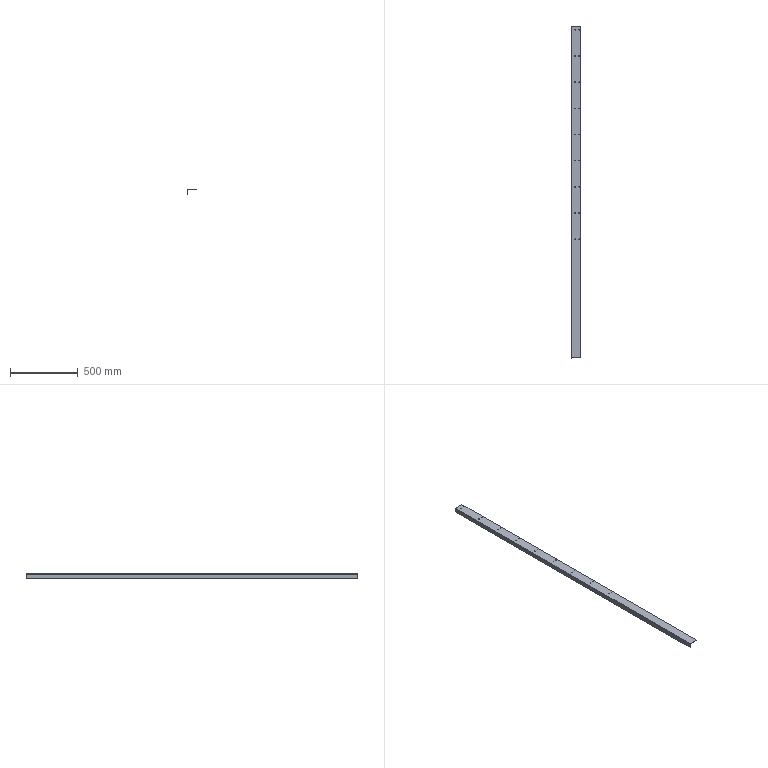Part | SolidWorks | features Cut 1, EdgeFlange 1, FlatPattern 1, ICE 1, SMBaseFlange 1, SheetMetal 1 | 1 solid | 50 faces | box 70 x 2448 x 32 mm | volume 293569 mm3 | cylinder 38 | plane 12 | commonest cylinder face diameters 4 x36 2.4 x1 4.8 x1